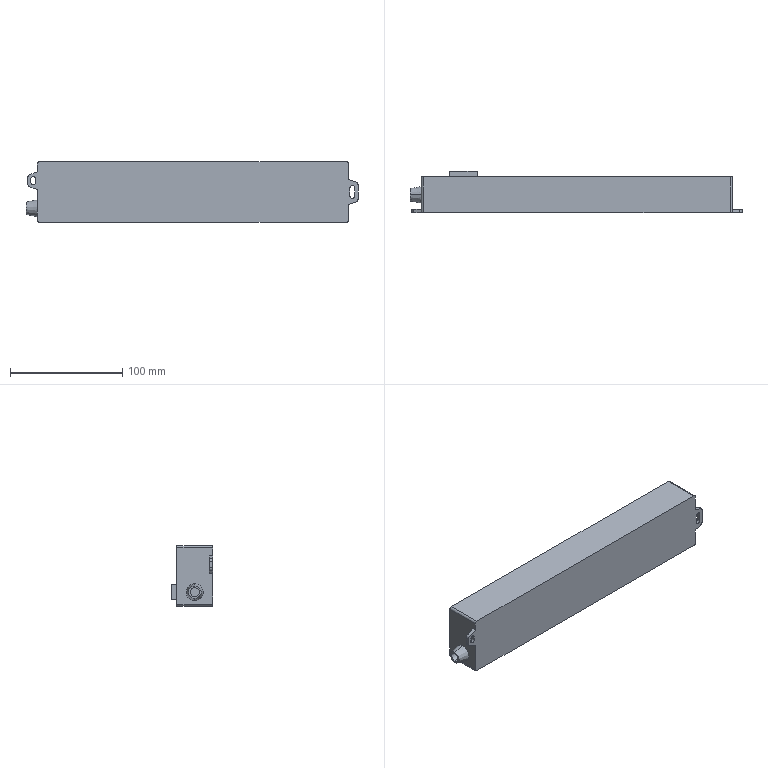Part | STEP file | 1 solid | 230 faces | box 295.5 x 37 x 54 mm | volume 476987 mm3 | plane 175 | cylinder 36 | spline 17 | cone 2 | commonest cylinder face diameters 4.618 x20 4.3 x6 4 x4 6 x4 8 x2